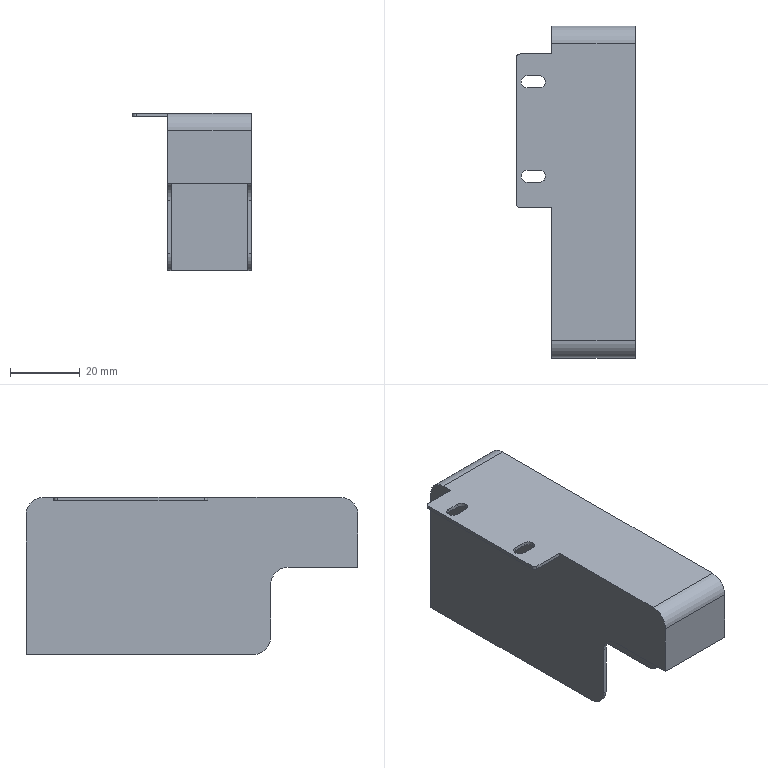Part | STEP file | 11-FG-B01211 | 1 solid | 38 faces | box 34 x 95 x 45 mm | volume 11150 mm3 | plane 22 | cylinder 16 | commonest cylinder face diameters 10 x8 3.5 x6 2 x2
STEP:
#1=CARTESIAN_POINT('',(-13.75,4.5,44.));
#2=VERTEX_POINT('',#1);
#3=CARTESIAN_POINT('',(-15.5,6.25,44.));
#4=VERTEX_POINT('',#3);
#5=CARTESIAN_POINT('',(-15.5,4.5,44.));
#6=DIRECTION('',(0.,0.,1.));
#7=DIRECTION('',(1.,0.,0.));
#8=AXIS2_PLACEMENT_3D('',#5,#6,#7);
#9=CIRCLE('',#8,1.75);
#10=EDGE_CURVE('',#2,#4,#9,.T.);
#11=ORIENTED_EDGE('',*,*,#10,.F.);
#12=CARTESIAN_POINT('',(-13.75,4.5,45.));
#13=VERTEX_POINT('',#12);
#14=CARTESIAN_POINT('',(-13.75,4.5,-20.));
#15=DIRECTION('',(0.,0.,1.));
#16=VECTOR('',#15,1000.);
#17=LINE('',#14,#16);
#18=EDGE_CURVE('',#2,#13,#17,.T.);
#19=ORIENTED_EDGE('',*,*,#18,.T.);
#20=CARTESIAN_POINT('',(-15.5,6.25,45.));
#21=VERTEX_POINT('',#20);
#22=CARTESIAN_POINT('',(-15.5,4.5,45.));
#23=DIRECTION('',(0.,0.,1.));
#24=DIRECTION('',(1.,0.,0.));
#25=AXIS2_PLACEMENT_3D('',#22,#23,#24);
#26=CIRCLE('',#25,1.75);
#27=EDGE_CURVE('',#13,#21,#26,.T.);
#28=ORIENTED_EDGE('',*,*,#27,.T.);
#29=CARTESIAN_POINT('',(-15.5,6.25,-20.));
#30=DIRECTION('',(0.,0.,1.));
#31=VECTOR('',#30,1000.);
#32=LINE('',#29,#31);
#33=EDGE_CURVE('',#4,#21,#32,.T.);
#34=ORIENTED_EDGE('',*,*,#33,.F.);
#35=EDGE_LOOP('',(#11,#19,#28,#34));
#36=FACE_OUTER_BOUND('',#35,.T.);
#37=CARTESIAN_POINT('',(-15.5,4.5,-20.));
#38=DIRECTION('',(0.,0.,1.));
#39=DIRECTION('',(1.,0.,0.));
#40=AXIS2_PLACEMENT_3D('',#37,#38,#39);
#41=CYLINDRICAL_SURFACE('',#40,1.75);
#42=ADVANCED_FACE('',(#36),#41,.F.);
#43=CARTESIAN_POINT('',(-13.75,31.5,44.));
#44=VERTEX_POINT('',#43);
#45=CARTESIAN_POINT('',(-15.5,33.25,44.));
#46=VERTEX_POINT('',#45);
#47=CARTESIAN_POINT('',(-15.5,31.5,44.));
#48=DIRECTION('',(0.,0.,1.));
#49=DIRECTION('',(1.,0.,0.));
#50=AXIS2_PLACEMENT_3D('',#47,#48,#49);
#51=CIRCLE('',#50,1.75);
#52=EDGE_CURVE('',#44,#46,#51,.T.);
#53=ORIENTED_EDGE('',*,*,#52,.F.);
#54=CARTESIAN_POINT('',(-13.75,31.5,45.));
#55=VERTEX_POINT('',#54);
#56=CARTESIAN_POINT('',(-13.75,31.5,-20.));
#57=DIRECTION('',(0.,0.,1.));
#58=VECTOR('',#57,1000.);
#59=LINE('',#56,#58);
#60=EDGE_CURVE('',#44,#55,#59,.T.);
#61=ORIENTED_EDGE('',*,*,#60,.T.);
#62=CARTESIAN_POINT('',(-15.5,33.25,45.));
#63=VERTEX_POINT('',#62);
#64=CARTESIAN_POINT('',(-15.5,31.5,45.));
#65=DIRECTION('',(0.,0.,1.));
#66=DIRECTION('',(1.,0.,0.));
#67=AXIS2_PLACEMENT_3D('',#64,#65,#66);
#68=CIRCLE('',#67,1.75);
#69=EDGE_CURVE('',#55,#63,#68,.T.);
#70=ORIENTED_EDGE('',*,*,#69,.T.);
#71=CARTESIAN_POINT('',(-15.5,33.25,-20.));
#72=DIRECTION('',(0.,0.,1.));
#73=VECTOR('',#72,1000.);
#74=LINE('',#71,#73);
#75=EDGE_CURVE('',#46,#63,#74,.T.);
#76=ORIENTED_EDGE('',*,*,#75,.F.);
#77=EDGE_LOOP('',(#53,#61,#70,#76));
#78=FACE_OUTER_BOUND('',#77,.T.);
#79=CARTESIAN_POINT('',(-15.5,31.5,-20.));
#80=DIRECTION('',(0.,0.,1.));
#81=DIRECTION('',(1.,0.,0.));
#82=AXIS2_PLACEMENT_3D('',#79,#80,#81);
#83=CYLINDRICAL_SURFACE('',#82,1.75);
#84=ADVANCED_FACE('',(#78),#83,.F.);
#85=CARTESIAN_POINT('',(-12.,47.5,0.));
#86=VERTEX_POINT('',#85);
#87=CARTESIAN_POINT('',(-12.,-17.5,0.));
#88=VERTEX_POINT('',#87);
#89=CARTESIAN_POINT('',(-12.,47.5,0.));
#90=DIRECTION('',(0.,-1.,0.));
#91=VECTOR('',#90,1000.);
#92=LINE('',#89,#91);
#93=EDGE_CURVE('',#86,#88,#92,.T.);
#94=ORIENTED_EDGE('',*,*,#93,.T.);
#95=CARTESIAN_POINT('',(-12.,-22.5,5.));
#96=VERTEX_POINT('',#95);
#97=CARTESIAN_POINT('',(-12.,-17.5,5.));
#98=DIRECTION('',(-1.,0.,0.));
#99=DIRECTION('',(0.,1.,0.));
#100=AXIS2_PLACEMENT_3D('',#97,#98,#99);
#101=CIRCLE('',#100,5.);
#102=EDGE_CURVE('',#88,#96,#101,.T.);
#103=ORIENTED_EDGE('',*,*,#102,.T.);
#104=CARTESIAN_POINT('',(-12.,-22.5,20.));
#105=VERTEX_POINT('',#104);
#106=CARTESIAN_POINT('',(-12.,-22.5,0.));
#107=DIRECTION('',(0.,0.,-1.));
#108=VECTOR('',#107,1000.);
#109=LINE('',#106,#108);
#110=EDGE_CURVE('',#105,#96,#109,.T.);
#111=ORIENTED_EDGE('',*,*,#110,.F.);
#112=CARTESIAN_POINT('',(-12.,-27.5,25.));
#113=VERTEX_POINT('',#112);
#114=CARTESIAN_POINT('',(-12.,-27.5,20.));
#115=DIRECTION('',(1.,0.,0.));
#116=DIRECTION('',(0.,1.,0.));
#117=AXIS2_PLACEMENT_3D('',#114,#115,#116);
#118=CIRCLE('',#117,5.);
#119=EDGE_CURVE('',#105,#113,#118,.T.);
#120=ORIENTED_EDGE('',*,*,#119,.T.);
#121=CARTESIAN_POINT('',(-12.,-47.5,25.));
#122=VERTEX_POINT('',#121);
#123=CARTESIAN_POINT('',(-12.,-47.5,25.));
#124=DIRECTION('',(0.,1.,0.));
#125=VECTOR('',#124,1000.);
#126=LINE('',#123,#125);
#127=EDGE_CURVE('',#122,#113,#126,.T.);
#128=ORIENTED_EDGE('',*,*,#127,.F.);
#129=CARTESIAN_POINT('',(-12.,-47.5,40.));
#130=VERTEX_POINT('',#129);
#131=CARTESIAN_POINT('',(-12.,-47.5,45.));
#132=DIRECTION('',(0.,0.,-1.));
#133=VECTOR('',#132,1000.);
#134=LINE('',#131,#133);
#135=EDGE_CURVE('',#130,#122,#134,.T.);
#136=ORIENTED_EDGE('',*,*,#135,.F.);
#137=CARTESIAN_POINT('',(-12.,-42.5,45.));
#138=VERTEX_POINT('',#137);
#139=CARTESIAN_POINT('',(-12.,-42.5,40.));
#140=DIRECTION('',(-1.,0.,0.));
#141=DIRECTION('',(0.,1.,0.));
#142=AXIS2_PLACEMENT_3D('',#139,#140,#141);
#143=CIRCLE('',#142,5.);
#144=EDGE_CURVE('',#130,#138,#143,.T.);
#145=ORIENTED_EDGE('',*,*,#144,.T.);
#146=CARTESIAN_POINT('',(-12.,-4.5,45.));
#147=VERTEX_POINT('',#146);
#148=CARTESIAN_POINT('',(-12.,47.5,45.));
#149=DIRECTION('',(0.,-1.,0.));
#150=VECTOR('',#149,1000.);
#151=LINE('',#148,#150);
#152=EDGE_CURVE('',#147,#138,#151,.T.);
#153=ORIENTED_EDGE('',*,*,#152,.F.);
#154=CARTESIAN_POINT('',(-12.,-4.5,44.));
#155=VERTEX_POINT('',#154);
#156=CARTESIAN_POINT('',(-12.,-4.5,-20.));
#157=DIRECTION('',(0.,0.,1.));
#158=VECTOR('',#157,1000.);
#159=LINE('',#156,#158);
#160=EDGE_CURVE('',#155,#147,#159,.T.);
#161=ORIENTED_EDGE('',*,*,#160,.F.);
#162=CARTESIAN_POINT('',(-12.,39.5,44.));
#163=VERTEX_POINT('',#162);
#164=CARTESIAN_POINT('',(-12.,47.5,44.));
#165=DIRECTION('',(0.,-1.,0.));
#166=VECTOR('',#165,1000.);
#167=LINE('',#164,#166);
#168=EDGE_CURVE('',#163,#155,#167,.T.);
#169=ORIENTED_EDGE('',*,*,#168,.F.);
#170=CARTESIAN_POINT('',(-12.,39.5,45.));
#171=VERTEX_POINT('',#170);
#172=CARTESIAN_POINT('',(-12.,39.5,109.));
#173=DIRECTION('',(0.,0.,-1.));
#174=VECTOR('',#173,1000.);
#175=LINE('',#172,#174);
#176=EDGE_CURVE('',#171,#163,#175,.T.);
#177=ORIENTED_EDGE('',*,*,#176,.F.);
#178=CARTESIAN_POINT('',(-12.,42.5,45.));
#179=VERTEX_POINT('',#178);
#180=CARTESIAN_POINT('',(-12.,0.,45.));
#181=DIRECTION('',(0.,1.,0.));
#182=VECTOR('',#181,1000.);
#183=LINE('',#180,#182);
#184=EDGE_CURVE('',#171,#179,#183,.T.);
#185=ORIENTED_EDGE('',*,*,#184,.T.);
#186=CARTESIAN_POINT('',(-12.,47.5,40.));
#187=VERTEX_POINT('',#186);
#188=CARTESIAN_POINT('',(-12.,42.5,40.));
#189=DIRECTION('',(-1.,0.,0.));
#190=DIRECTION('',(0.,1.,0.));
#191=AXIS2_PLACEMENT_3D('',#188,#189,#190);
#192=CIRCLE('',#191,5.);
#193=EDGE_CURVE('',#179,#187,#192,.T.);
#194=ORIENTED_EDGE('',*,*,#193,.T.);
#195=CARTESIAN_POINT('',(-12.,47.5,45.));
#196=DIRECTION('',(0.,0.,-1.));
#197=VECTOR('',#196,1000.);
#198=LINE('',#195,#197);
#199=EDGE_CURVE('',#187,#86,#198,.T.);
#200=ORIENTED_EDGE('',*,*,#199,.T.);
#201=EDGE_LOOP('',(#94,#103,#111,#120,#128,#136,#145,#153,#161,#169,#177,#185,#194,#200));
#202=FACE_OUTER_BOUND('',#201,.T.);
#203=CARTESIAN_POINT('',(-12.,47.5,45.));
#204=DIRECTION('',(1.,0.,0.));
#205=DIRECTION('',(0.,1.,0.));
#206=AXIS2_PLACEMENT_3D('',#203,#204,#205);
#207=PLANE('',#206);
#208=ADVANCED_FACE('',(#202),#207,.F.);
#209=CARTESIAN_POINT('',(12.,-22.5,20.));
#210=VERTEX_POINT('',#209);
#211=CARTESIAN_POINT('',(12.,-22.5,5.));
#212=VERTEX_POINT('',#211);
#213=CARTESIAN_POINT('',(12.,-22.5,45.));
#214=DIRECTION('',(0.,0.,-1.));
#215=VECTOR('',#214,1000.);
#216=LINE('',#213,#215);
#217=EDGE_CURVE('',#210,#212,#216,.T.);
#218=ORIENTED_EDGE('',*,*,#217,.T.);
#219=CARTESIAN_POINT('',(12.,-17.5,0.));
#220=VERTEX_POINT('',#219);
#221=CARTESIAN_POINT('',(12.,-17.5,5.));
#222=DIRECTION('',(1.,0.,0.));
#223=DIRECTION('',(0.,-1.,0.));
#224=AXIS2_PLACEMENT_3D('',#221,#222,#223);
#225=CIRCLE('',#224,5.);
#226=EDGE_CURVE('',#212,#220,#225,.T.);
#227=ORIENTED_EDGE('',*,*,#226,.T.);
#228=CARTESIAN_POINT('',(12.,47.5,0.));
#229=VERTEX_POINT('',#228);
#230=CARTESIAN_POINT('',(12.,47.5,0.));
#231=DIRECTION('',(0.,1.,0.));
#232=VECTOR('',#231,1000.);
#233=LINE('',#230,#232);
#234=EDGE_CURVE('',#220,#229,#233,.T.);
#235=ORIENTED_EDGE('',*,*,#234,.T.);
#236=CARTESIAN_POINT('',(12.,47.5,40.));
#237=VERTEX_POINT('',#236);
#238=CARTESIAN_POINT('',(12.,47.5,45.));
#239=DIRECTION('',(0.,0.,-1.));
#240=VECTOR('',#239,1000.);
#241=LINE('',#238,#240);
#242=EDGE_CURVE('',#237,#229,#241,.T.);
#243=ORIENTED_EDGE('',*,*,#242,.F.);
#244=CARTESIAN_POINT('',(12.,42.5,45.));
#245=VERTEX_POINT('',#244);
#246=CARTESIAN_POINT('',(12.,42.5,40.));
#247=DIRECTION('',(1.,0.,0.));
#248=DIRECTION('',(0.,-1.,0.));
#249=AXIS2_PLACEMENT_3D('',#246,#247,#248);
#250=CIRCLE('',#249,5.);
#251=EDGE_CURVE('',#237,#245,#250,.T.);
#252=ORIENTED_EDGE('',*,*,#251,.T.);
#253=CARTESIAN_POINT('',(12.,-42.5,45.));
#254=VERTEX_POINT('',#253);
#255=CARTESIAN_POINT('',(12.,47.5,45.));
#256=DIRECTION('',(0.,1.,0.));
#257=VECTOR('',#256,1000.);
#258=LINE('',#255,#257);
#259=EDGE_CURVE('',#254,#245,#258,.T.);
#260=ORIENTED_EDGE('',*,*,#259,.F.);
#261=CARTESIAN_POINT('',(12.,-47.5,40.));
#262=VERTEX_POINT('',#261);
#263=CARTESIAN_POINT('',(12.,-42.5,40.));
#264=DIRECTION('',(1.,0.,0.));
#265=DIRECTION('',(0.,-1.,0.));
#266=AXIS2_PLACEMENT_3D('',#263,#264,#265);
#267=CIRCLE('',#266,5.);
#268=EDGE_CURVE('',#254,#262,#267,.T.);
#269=ORIENTED_EDGE('',*,*,#268,.T.);
#270=CARTESIAN_POINT('',(12.,-47.5,25.));
#271=VERTEX_POINT('',#270);
#272=CARTESIAN_POINT('',(12.,-47.5,45.));
#273=DIRECTION('',(0.,0.,-1.));
#274=VECTOR('',#273,1000.);
#275=LINE('',#272,#274);
#276=EDGE_CURVE('',#262,#271,#275,.T.);
#277=ORIENTED_EDGE('',*,*,#276,.T.);
#278=CARTESIAN_POINT('',(12.,-27.5,25.));
#279=VERTEX_POINT('',#278);
#280=CARTESIAN_POINT('',(12.,47.5,25.));
#281=DIRECTION('',(0.,1.,0.));
#282=VECTOR('',#281,1000.);
#283=LINE('',#280,#282);
#284=EDGE_CURVE('',#271,#279,#283,.T.);
#285=ORIENTED_EDGE('',*,*,#284,.T.);
#286=CARTESIAN_POINT('',(12.,-27.5,20.));
#287=DIRECTION('',(-1.,0.,0.));
#288=DIRECTION('',(0.,-1.,0.));
#289=AXIS2_PLACEMENT_3D('',#286,#287,#288);
#290=CIRCLE('',#289,5.);
#291=EDGE_CURVE('',#279,#210,#290,.T.);
#292=ORIENTED_EDGE('',*,*,#291,.T.);
#293=EDGE_LOOP('',(#218,#227,#235,#243,#252,#260,#269,#277,#285,#292));
#294=FACE_OUTER_BOUND('',#293,.T.);
#295=CARTESIAN_POINT('',(12.,47.5,45.));
#296=DIRECTION('',(-1.,0.,0.));
#297=DIRECTION('',(0.,-1.,0.));
#298=AXIS2_PLACEMENT_3D('',#295,#296,#297);
#299=PLANE('',#298);
#300=ADVANCED_FACE('',(#294),#299,.F.);
#301=ORIENTED_EDGE('',*,*,#199,.F.);
#302=CARTESIAN_POINT('',(12.,47.5,40.));
#303=DIRECTION('',(1.,0.,0.));
#304=VECTOR('',#303,1000.);
#305=LINE('',#302,#304);
#306=EDGE_CURVE('',#187,#237,#305,.T.);
#307=ORIENTED_EDGE('',*,*,#306,.T.);
#308=ORIENTED_EDGE('',*,*,#242,.T.);
#309=CARTESIAN_POINT('',(-12.,47.5,0.));
#310=DIRECTION('',(-1.,0.,0.));
#311=VECTOR('',#310,1000.);
#312=LINE('',#309,#311);
#313=EDGE_CURVE('',#229,#86,#312,.T.);
#314=ORIENTED_EDGE('',*,*,#313,.T.);
#315=EDGE_LOOP('',(#301,#307,#308,#314));
#316=FACE_OUTER_BOUND('',#315,.T.);
#317=CARTESIAN_POINT('',(-12.,47.5,45.));
#318=DIRECTION('',(0.,-1.,0.));
#319=DIRECTION('',(0.,0.,-1.));
#320=AXIS2_PLACEMENT_3D('',#317,#318,#319);
#321=PLANE('',#320);
#322=ADVANCED_FACE('',(#316),#321,.F.);
#323=ORIENTED_EDGE('',*,*,#135,.T.);
#324=CARTESIAN_POINT('',(53.,-47.5,25.));
#325=DIRECTION('',(-1.,0.,0.));
#326=VECTOR('',#325,1000.);
#327=LINE('',#324,#326);
#328=EDGE_CURVE('',#271,#122,#327,.T.);
#329=ORIENTED_EDGE('',*,*,#328,.F.);
#330=ORIENTED_EDGE('',*,*,#276,.F.);
#331=CARTESIAN_POINT('',(-12.,-47.5,40.));
#332=DIRECTION('',(-1.,0.,0.));
#333=VECTOR('',#332,1000.);
#334=LINE('',#331,#333);
#335=EDGE_CURVE('',#262,#130,#334,.T.);
#336=ORIENTED_EDGE('',*,*,#335,.T.);
#337=EDGE_LOOP('',(#323,#329,#330,#336));
#338=FACE_OUTER_BOUND('',#337,.T.);
#339=CARTESIAN_POINT('',(-12.,-47.5,45.));
#340=DIRECTION('',(0.,1.,0.));
#341=DIRECTION('',(0.,0.,1.));
#342=AXIS2_PLACEMENT_3D('',#339,#340,#341);
#343=PLANE('',#342);
#344=ADVANCED_FACE('',(#338),#343,.F.);
#345=CARTESIAN_POINT('',(-22.,38.5,45.));
#346=VERTEX_POINT('',#345);
#347=CARTESIAN_POINT('',(-22.,-3.5,45.));
#348=VERTEX_POINT('',#347);
#349=CARTESIAN_POINT('',(-22.,47.5,45.));
#350=DIRECTION('',(0.,-1.,0.));
#351=VECTOR('',#350,1000.);
#352=LINE('',#349,#351);
#353=EDGE_CURVE('',#346,#348,#352,.T.);
#354=ORIENTED_EDGE('',*,*,#353,.T.);
#355=CARTESIAN_POINT('',(-21.,-4.5,45.));
#356=VERTEX_POINT('',#355);
#357=CARTESIAN_POINT('',(-21.,-3.5,45.));
#358=DIRECTION('',(0.,0.,1.));
#359=DIRECTION('',(1.,0.,0.));
#360=AXIS2_PLACEMENT_3D('',#357,#358,#359);
#361=CIRCLE('',#360,1.);
#362=EDGE_CURVE('',#348,#356,#361,.T.);
#363=ORIENTED_EDGE('',*,*,#362,.T.);
#364=CARTESIAN_POINT('',(-12.,-4.5,45.));
#365=DIRECTION('',(-1.,0.,0.));
#366=VECTOR('',#365,1000.);
#367=LINE('',#364,#366);
#368=EDGE_CURVE('',#147,#356,#367,.T.);
#369=ORIENTED_EDGE('',*,*,#368,.F.);
#370=ORIENTED_EDGE('',*,*,#152,.T.);
#371=CARTESIAN_POINT('',(12.,-42.5,45.));
#372=DIRECTION('',(1.,0.,0.));
#373=VECTOR('',#372,1000.);
#374=LINE('',#371,#373);
#375=EDGE_CURVE('',#138,#254,#374,.T.);
#376=ORIENTED_EDGE('',*,*,#375,.T.);
#377=ORIENTED_EDGE('',*,*,#259,.T.);
#378=CARTESIAN_POINT('',(-22.,42.5,45.));
#379=DIRECTION('',(-1.,0.,0.));
#380=VECTOR('',#379,1000.);
#381=LINE('',#378,#380);
#382=EDGE_CURVE('',#245,#179,#381,.T.);
#383=ORIENTED_EDGE('',*,*,#382,.T.);
#384=ORIENTED_EDGE('',*,*,#184,.F.);
#385=CARTESIAN_POINT('',(-21.,39.5,45.));
#386=VERTEX_POINT('',#385);
#387=CARTESIAN_POINT('',(0.,39.5,45.));
#388=DIRECTION('',(1.,0.,0.));
#389=VECTOR('',#388,1000.);
#390=LINE('',#387,#389);
#391=EDGE_CURVE('',#386,#171,#390,.T.);
#392=ORIENTED_EDGE('',*,*,#391,.F.);
#393=CARTESIAN_POINT('',(-21.,38.5,45.));
#394=DIRECTION('',(0.,0.,1.));
#395=DIRECTION('',(1.,0.,0.));
#396=AXIS2_PLACEMENT_3D('',#393,#394,#395);
#397=CIRCLE('',#396,1.);
#398=EDGE_CURVE('',#386,#346,#397,.T.);
#399=ORIENTED_EDGE('',*,*,#398,.T.);
#400=EDGE_LOOP('',(#354,#363,#369,#370,#376,#377,#383,#384,#392,#399));
#401=FACE_OUTER_BOUND('',#400,.T.);
#402=CARTESIAN_POINT('',(-19.,6.25,45.));
#403=VERTEX_POINT('',#402);
#404=CARTESIAN_POINT('',(-19.,2.75,45.));
#405=VERTEX_POINT('',#404);
#406=CARTESIAN_POINT('',(-19.,4.5,45.));
#407=DIRECTION('',(0.,0.,1.));
#408=DIRECTION('',(1.,0.,0.));
#409=AXIS2_PLACEMENT_3D('',#406,#407,#408);
#410=CIRCLE('',#409,1.75);
#411=EDGE_CURVE('',#403,#405,#410,.T.);
#412=ORIENTED_EDGE('',*,*,#411,.F.);
#413=CARTESIAN_POINT('',(-19.,6.25,45.));
#414=DIRECTION('',(-1.,0.,0.));
#415=VECTOR('',#414,1000.);
#416=LINE('',#413,#415);
#417=EDGE_CURVE('',#21,#403,#416,.T.);
#418=ORIENTED_EDGE('',*,*,#417,.F.);
#419=ORIENTED_EDGE('',*,*,#27,.F.);
#420=CARTESIAN_POINT('',(-15.5,2.75,45.));
#421=VERTEX_POINT('',#420);
#422=CARTESIAN_POINT('',(-15.5,4.5,45.));
#423=DIRECTION('',(0.,0.,1.));
#424=DIRECTION('',(1.,0.,0.));
#425=AXIS2_PLACEMENT_3D('',#422,#423,#424);
#426=CIRCLE('',#425,1.75);
#427=EDGE_CURVE('',#421,#13,#426,.T.);
#428=ORIENTED_EDGE('',*,*,#427,.F.);
#429=CARTESIAN_POINT('',(-19.,2.75,45.));
#430=DIRECTION('',(1.,0.,0.));
#431=VECTOR('',#430,1000.);
#432=LINE('',#429,#431);
#433=EDGE_CURVE('',#405,#421,#432,.T.);
#434=ORIENTED_EDGE('',*,*,#433,.F.);
#435=EDGE_LOOP('',(#412,#418,#419,#428,#434));
#436=FACE_BOUND('',#435,.T.);
#437=CARTESIAN_POINT('',(-19.,33.25,45.));
#438=VERTEX_POINT('',#437);
#439=CARTESIAN_POINT('',(-19.,29.75,45.));
#440=VERTEX_POINT('',#439);
#441=CARTESIAN_POINT('',(-19.,31.5,45.));
#442=DIRECTION('',(0.,0.,1.));
#443=DIRECTION('',(1.,0.,0.));
#444=AXIS2_PLACEMENT_3D('',#441,#442,#443);
#445=CIRCLE('',#444,1.75);
#446=EDGE_CURVE('',#438,#440,#445,.T.);
#447=ORIENTED_EDGE('',*,*,#446,.F.);
#448=CARTESIAN_POINT('',(-19.,33.25,45.));
#449=DIRECTION('',(-1.,0.,0.));
#450=VECTOR('',#449,1000.);
#451=LINE('',#448,#450);
#452=EDGE_CURVE('',#63,#438,#451,.T.);
#453=ORIENTED_EDGE('',*,*,#452,.F.);
#454=ORIENTED_EDGE('',*,*,#69,.F.);
#455=CARTESIAN_POINT('',(-15.5,29.75,45.));
#456=VERTEX_POINT('',#455);
#457=CARTESIAN_POINT('',(-15.5,31.5,45.));
#458=DIRECTION('',(0.,0.,1.));
#459=DIRECTION('',(1.,0.,0.));
#460=AXIS2_PLACEMENT_3D('',#457,#458,#459);
#461=CIRCLE('',#460,1.75);
#462=EDGE_CURVE('',#456,#55,#461,.T.);
#463=ORIENTED_EDGE('',*,*,#462,.F.);
#464=CARTESIAN_POINT('',(-19.,29.75,45.));
#465=DIRECTION('',(1.,0.,0.));
#466=VECTOR('',#465,1000.);
#467=LINE('',#464,#466);
#468=EDGE_CURVE('',#440,#456,#467,.T.);
#469=ORIENTED_EDGE('',*,*,#468,.F.);
#470=EDGE_LOOP('',(#447,#453,#454,#463,#469));
#471=FACE_BOUND('',#470,.T.);
#472=CARTESIAN_POINT('',(0.,0.,45.));
#473=DIRECTION('',(0.,0.,1.));
#474=DIRECTION('',(1.,0.,0.));
#475=AXIS2_PLACEMENT_3D('',#472,#473,#474);
#476=PLANE('',#475);
#477=ADVANCED_FACE('',(#401,#436,#471),#476,.T.);
#478=ORIENTED_EDGE('',*,*,#234,.F.);
#479=CARTESIAN_POINT('',(11.,-17.5,0.));
#480=VERTEX_POINT('',#479);
#481=CARTESIAN_POINT('',(0.,-17.5,0.));
#482=DIRECTION('',(-1.,0.,0.));
#483=VECTOR('',#482,1000.);
#484=LINE('',#481,#483);
#485=EDGE_CURVE('',#220,#480,#484,.T.);
#486=ORIENTED_EDGE('',*,*,#485,.T.);
#487=CARTESIAN_POINT('',(11.,46.5,0.));
#488=VERTEX_POINT('',#487);
#489=CARTESIAN_POINT('',(11.,47.5,0.));
#490=DIRECTION('',(0.,1.,0.));
#491=VECTOR('',#490,1000.);
#492=LINE('',#489,#491);
#493=EDGE_CURVE('',#480,#488,#492,.T.);
#494=ORIENTED_EDGE('',*,*,#493,.T.);
#495=CARTESIAN_POINT('',(-11.,46.5,0.));
#496=VERTEX_POINT('',#495);
#497=CARTESIAN_POINT('',(-12.,46.5,0.));
#498=DIRECTION('',(-1.,0.,0.));
#499=VECTOR('',#498,1000.);
#500=LINE('',#497,#499);
#501=EDGE_CURVE('',#488,#496,#500,.T.);
#502=ORIENTED_EDGE('',*,*,#501,.T.);
#503=CARTESIAN_POINT('',(-11.,-17.5,0.));
#504=VERTEX_POINT('',#503);
#505=CARTESIAN_POINT('',(-11.,47.5,0.));
#506=DIRECTION('',(0.,-1.,0.));
#507=VECTOR('',#506,1000.);
#508=LINE('',#505,#507);
#509=EDGE_CURVE('',#496,#504,#508,.T.);
#510=ORIENTED_EDGE('',*,*,#509,.T.);
#511=CARTESIAN_POINT('',(0.,-17.5,0.));
#512=DIRECTION('',(-1.,0.,0.));
#513=VECTOR('',#512,1000.);
#514=LINE('',#511,#513);
#515=EDGE_CURVE('',#504,#88,#514,.T.);
#516=ORIENTED_EDGE('',*,*,#515,.T.);
#517=ORIENTED_EDGE('',*,*,#93,.F.);
#518=ORIENTED_EDGE('',*,*,#313,.F.);
#519=EDGE_LOOP('',(#478,#486,#494,#502,#510,#516,#517,#518));
#520=FACE_OUTER_BOUND('',#519,.T.);
#521=CARTESIAN_POINT('',(0.,0.,0.));
#522=DIRECTION('',(0.,0.,1.));
#523=DIRECTION('',(1.,0.,0.));
#524=AXIS2_PLACEMENT_3D('',#521,#522,#523);
#525=PLANE('',#524);
#526=ADVANCED_FACE('',(#520),#525,.F.);
#527=ORIENTED_EDGE('',*,*,#493,.F.);
#528=CARTESIAN_POINT('',(11.,-22.5,5.));
#529=VERTEX_POINT('',#528);
#530=CARTESIAN_POINT('',(11.,-17.5,5.));
#531=DIRECTION('',(-1.,0.,0.));
#532=DIRECTION('',(0.,-1.,0.));
#533=AXIS2_PLACEMENT_3D('',#530,#531,#532);
#534=CIRCLE('',#533,5.);
#535=EDGE_CURVE('',#480,#529,#534,.T.);
#536=ORIENTED_EDGE('',*,*,#535,.T.);
#537=CARTESIAN_POINT('',(11.,-22.5,20.));
#538=VERTEX_POINT('',#537);
#539=CARTESIAN_POINT('',(11.,-22.5,45.));
#540=DIRECTION('',(0.,0.,-1.));
#541=VECTOR('',#540,1000.);
#542=LINE('',#539,#541);
#543=EDGE_CURVE('',#538,#529,#542,.T.);
#544=ORIENTED_EDGE('',*,*,#543,.F.);
#545=CARTESIAN_POINT('',(11.,-27.5,25.));
#546=VERTEX_POINT('',#545);
#547=CARTESIAN_POINT('',(11.,-27.5,20.));
#548=DIRECTION('',(1.,0.,0.));
#549=DIRECTION('',(0.,-1.,0.));
#550=AXIS2_PLACEMENT_3D('',#547,#548,#549);
#551=CIRCLE('',#550,5.);
#552=EDGE_CURVE('',#538,#546,#551,.T.);
#553=ORIENTED_EDGE('',*,*,#552,.T.);
#554=CARTESIAN_POINT('',(11.,-46.5,25.));
#555=VERTEX_POINT('',#554);
#556=CARTESIAN_POINT('',(11.,47.5,25.));
#557=DIRECTION('',(0.,1.,0.));
#558=VECTOR('',#557,1000.);
#559=LINE('',#556,#558);
#560=EDGE_CURVE('',#555,#546,#559,.T.);
#561=ORIENTED_EDGE('',*,*,#560,.F.);
#562=CARTESIAN_POINT('',(11.,-46.5,39.));
#563=VERTEX_POINT('',#562);
#564=CARTESIAN_POINT('',(11.,-46.5,45.));
#565=DIRECTION('',(0.,0.,-1.));
#566=VECTOR('',#565,1000.);
#567=LINE('',#564,#566);
#568=EDGE_CURVE('',#563,#555,#567,.T.);
#569=ORIENTED_EDGE('',*,*,#568,.F.);
#570=CARTESIAN_POINT('',(11.,-41.5,44.));
#571=VERTEX_POINT('',#570);
#572=CARTESIAN_POINT('',(11.,-41.5,39.));
#573=DIRECTION('',(-1.,0.,0.));
#574=DIRECTION('',(0.,-1.,0.));
#575=AXIS2_PLACEMENT_3D('',#572,#573,#574);
#576=CIRCLE('',#575,5.);
#577=EDGE_CURVE('',#563,#571,#576,.T.);
#578=ORIENTED_EDGE('',*,*,#577,.T.);
#579=CARTESIAN_POINT('',(11.,41.5,44.));
#580=VERTEX_POINT('',#579);
#581=CARTESIAN_POINT('',(11.,47.5,44.));
#582=DIRECTION('',(0.,1.,0.));
#583=VECTOR('',#582,1000.);
#584=LINE('',#581,#583);
#585=EDGE_CURVE('',#571,#580,#584,.T.);
#586=ORIENTED_EDGE('',*,*,#585,.T.);
#587=CARTESIAN_POINT('',(11.,46.5,39.));
#588=VERTEX_POINT('',#587);
#589=CARTESIAN_POINT('',(11.,41.5,39.));
#590=DIRECTION('',(-1.,0.,0.));
#591=DIRECTION('',(0.,-1.,0.));
#592=AXIS2_PLACEMENT_3D('',#589,#590,#591);
#593=CIRCLE('',#592,5.);
#594=EDGE_CURVE('',#580,#588,#593,.T.);
#595=ORIENTED_EDGE('',*,*,#594,.T.);
#596=CARTESIAN_POINT('',(11.,46.5,45.));
#597=DIRECTION('',(0.,0.,-1.));
#598=VECTOR('',#597,1000.);
#599=LINE('',#596,#598);
#600=EDGE_CURVE('',#588,#488,#599,.T.);
#601=ORIENTED_EDGE('',*,*,#600,.T.);
#602=EDGE_LOOP('',(#527,#536,#544,#553,#561,#569,#578,#586,#595,#601));
#603=FACE_OUTER_BOUND('',#602,.T.);
#604=CARTESIAN_POINT('',(11.,47.5,45.));
#605=DIRECTION('',(-1.,0.,0.));
#606=DIRECTION('',(0.,-1.,0.));
#607=AXIS2_PLACEMENT_3D('',#604,#605,#606);
#608=PLANE('',#607);
#609=ADVANCED_FACE('',(#603),#608,.T.);
#610=ORIENTED_EDGE('',*,*,#600,.F.);
#611=CARTESIAN_POINT('',(-11.,46.5,39.));
#612=VERTEX_POINT('',#611);
#613=CARTESIAN_POINT('',(-12.,46.5,39.));
#614=DIRECTION('',(-1.,0.,0.));
#615=VECTOR('',#614,1000.);
#616=LINE('',#613,#615);
#617=EDGE_CURVE('',#588,#612,#616,.T.);
#618=ORIENTED_EDGE('',*,*,#617,.T.);
#619=CARTESIAN_POINT('',(-11.,46.5,45.));
#620=DIRECTION('',(0.,0.,-1.));
#621=VECTOR('',#620,1000.);
#622=LINE('',#619,#621);
#623=EDGE_CURVE('',#612,#496,#622,.T.);
#624=ORIENTED_EDGE('',*,*,#623,.T.);
#625=ORIENTED_EDGE('',*,*,#501,.F.);
#626=EDGE_LOOP('',(#610,#618,#624,#625));
#627=FACE_OUTER_BOUND('',#626,.T.);
#628=CARTESIAN_POINT('',(-12.,46.5,45.));
#629=DIRECTION('',(0.,-1.,0.));
#630=DIRECTION('',(0.,0.,-1.));
#631=AXIS2_PLACEMENT_3D('',#628,#629,#630);
#632=PLANE('',#631);
#633=ADVANCED_FACE('',(#627),#632,.T.);
#634=CARTESIAN_POINT('',(-11.,-22.5,5.));
#635=VERTEX_POINT('',#634);
#636=CARTESIAN_POINT('',(-11.,-22.5,20.));
#637=VERTEX_POINT('',#636);
#638=CARTESIAN_POINT('',(-11.,-22.5,45.));
#639=DIRECTION('',(0.,0.,1.));
#640=VECTOR('',#639,1000.);
#641=LINE('',#638,#640);
#642=EDGE_CURVE('',#635,#637,#641,.T.);
#643=ORIENTED_EDGE('',*,*,#642,.F.);
#644=CARTESIAN_POINT('',(-11.,-17.5,5.));
#645=DIRECTION('',(1.,0.,0.));
#646=DIRECTION('',(0.,1.,0.));
#647=AXIS2_PLACEMENT_3D('',#644,#645,#646);
#648=CIRCLE('',#647,5.);
#649=EDGE_CURVE('',#635,#504,#648,.T.);
#650=ORIENTED_EDGE('',*,*,#649,.T.);
#651=ORIENTED_EDGE('',*,*,#509,.F.);
#652=ORIENTED_EDGE('',*,*,#623,.F.);
#653=CARTESIAN_POINT('',(-11.,41.5,44.));
#654=VERTEX_POINT('',#653);
#655=CARTESIAN_POINT('',(-11.,41.5,39.));
#656=DIRECTION('',(1.,0.,0.));
#657=DIRECTION('',(0.,1.,0.));
#658=AXIS2_PLACEMENT_3D('',#655,#656,#657);
#659=CIRCLE('',#658,5.);
#660=EDGE_CURVE('',#612,#654,#659,.T.);
#661=ORIENTED_EDGE('',*,*,#660,.T.);
#662=CARTESIAN_POINT('',(-11.,-41.5,44.));
#663=VERTEX_POINT('',#662);
#664=CARTESIAN_POINT('',(-11.,47.5,44.));
#665=DIRECTION('',(0.,-1.,0.));
#666=VECTOR('',#665,1000.);
#667=LINE('',#664,#666);
#668=EDGE_CURVE('',#654,#663,#667,.T.);
#669=ORIENTED_EDGE('',*,*,#668,.T.);
#670=CARTESIAN_POINT('',(-11.,-46.5,39.));
#671=VERTEX_POINT('',#670);
#672=CARTESIAN_POINT('',(-11.,-41.5,39.));
#673=DIRECTION('',(1.,0.,0.));
#674=DIRECTION('',(0.,1.,0.));
#675=AXIS2_PLACEMENT_3D('',#672,#673,#674);
#676=CIRCLE('',#675,5.);
#677=EDGE_CURVE('',#663,#671,#676,.T.);
#678=ORIENTED_EDGE('',*,*,#677,.T.);
#679=CARTESIAN_POINT('',(-11.,-46.5,25.));
#680=VERTEX_POINT('',#679);
#681=CARTESIAN_POINT('',(-11.,-46.5,45.));
#682=DIRECTION('',(0.,0.,-1.));
#683=VECTOR('',#682,1000.);
#684=LINE('',#681,#683);
#685=EDGE_CURVE('',#671,#680,#684,.T.);
#686=ORIENTED_EDGE('',*,*,#685,.T.);
#687=CARTESIAN_POINT('',(-11.,-27.5,25.));
#688=VERTEX_POINT('',#687);
#689=CARTESIAN_POINT('',(-11.,47.5,25.));
#690=DIRECTION('',(0.,-1.,0.));
#691=VECTOR('',#690,1000.);
#692=LINE('',#689,#691);
#693=EDGE_CURVE('',#688,#680,#692,.T.);
#694=ORIENTED_EDGE('',*,*,#693,.F.);
#695=CARTESIAN_POINT('',(-11.,-27.5,20.));
#696=DIRECTION('',(-1.,0.,0.));
#697=DIRECTION('',(0.,1.,0.));
#698=AXIS2_PLACEMENT_3D('',#695,#696,#697);
#699=CIRCLE('',#698,5.);
#700=EDGE_CURVE('',#688,#637,#699,.T.);
#701=ORIENTED_EDGE('',*,*,#700,.T.);
#702=EDGE_LOOP('',(#643,#650,#651,#652,#661,#669,#678,#686,#694,#701));
#703=FACE_OUTER_BOUND('',#702,.T.);
#704=CARTESIAN_POINT('',(-11.,47.5,45.));
#705=DIRECTION('',(1.,0.,0.));
#706=DIRECTION('',(0.,1.,0.));
#707=AXIS2_PLACEMENT_3D('',#704,#705,#706);
#708=PLANE('',#707);
#709=ADVANCED_FACE('',(#703),#708,.T.);
#710=CARTESIAN_POINT('',(-12.,-46.5,25.));
#711=DIRECTION('',(1.,0.,0.));
#712=VECTOR('',#711,1000.);
#713=LINE('',#710,#712);
#714=EDGE_CURVE('',#680,#555,#713,.T.);
#715=ORIENTED_EDGE('',*,*,#714,.F.);
#716=ORIENTED_EDGE('',*,*,#685,.F.);
#717=CARTESIAN_POINT('',(-12.,-46.5,39.));
#718=DIRECTION('',(1.,0.,0.));
#719=VECTOR('',#718,1000.);
#720=LINE('',#717,#719);
#721=EDGE_CURVE('',#671,#563,#720,.T.);
#722=ORIENTED_EDGE('',*,*,#721,.T.);
#723=ORIENTED_EDGE('',*,*,#568,.T.);
#724=EDGE_LOOP('',(#715,#716,#722,#723));
#725=FACE_OUTER_BOUND('',#724,.T.);
#726=CARTESIAN_POINT('',(-12.,-46.5,45.));
#727=DIRECTION('',(0.,1.,0.));
#728=DIRECTION('',(0.,0.,1.));
#729=AXIS2_PLACEMENT_3D('',#726,#727,#728);
#730=PLANE('',#729);
#731=ADVANCED_FACE('',(#725),#730,.T.);
#732=ORIENTED_EDGE('',*,*,#585,.F.);
#733=CARTESIAN_POINT('',(0.,-41.5,44.));
#734=DIRECTION('',(-1.,0.,0.));
#735=VECTOR('',#734,1000.);
#736=LINE('',#733,#735);
#737=EDGE_CURVE('',#571,#663,#736,.T.);
#738=ORIENTED_EDGE('',*,*,#737,.T.);
#739=ORIENTED_EDGE('',*,*,#668,.F.);
#740=CARTESIAN_POINT('',(0.,41.5,44.));
#741=DIRECTION('',(1.,0.,0.));
#742=VECTOR('',#741,1000.);
#743=LINE('',#740,#742);
#744=EDGE_CURVE('',#654,#580,#743,.T.);
#745=ORIENTED_EDGE('',*,*,#744,.T.);
#746=EDGE_LOOP('',(#732,#738,#739,#745));
#747=FACE_OUTER_BOUND('',#746,.T.);
#748=CARTESIAN_POINT('',(0.,0.,44.));
#749=DIRECTION('',(0.,0.,1.));
#750=DIRECTION('',(1.,0.,0.));
#751=AXIS2_PLACEMENT_3D('',#748,#749,#750);
#752=PLANE('',#751);
#753=ADVANCED_FACE('',(#747),#752,.F.);
#754=CARTESIAN_POINT('',(-19.,6.25,44.));
#755=VERTEX_POINT('',#754);
#756=CARTESIAN_POINT('',(-82.008,6.25,44.));
#757=DIRECTION('',(-1.,0.,0.));
#758=VECTOR('',#757,1000.);
#759=LINE('',#756,#758);
#760=EDGE_CURVE('',#4,#755,#759,.T.);
#761=ORIENTED_EDGE('',*,*,#760,.T.);
#762=CARTESIAN_POINT('',(-19.,2.75,44.));
#763=VERTEX_POINT('',#762);
#764=CARTESIAN_POINT('',(-19.,4.5,44.));
#765=DIRECTION('',(0.,0.,1.));
#766=DIRECTION('',(1.,0.,0.));
#767=AXIS2_PLACEMENT_3D('',#764,#765,#766);
#768=CIRCLE('',#767,1.75);
#769=EDGE_CURVE('',#755,#763,#768,.T.);
#770=ORIENTED_EDGE('',*,*,#769,.T.);
#771=CARTESIAN_POINT('',(-15.5,2.75,44.));
#772=VERTEX_POINT('',#771);
#773=CARTESIAN_POINT('',(-82.008,2.75,44.));
#774=DIRECTION('',(1.,0.,0.));
#775=VECTOR('',#774,1000.);
#776=LINE('',#773,#775);
#777=EDGE_CURVE('',#763,#772,#776,.T.);
#778=ORIENTED_EDGE('',*,*,#777,.T.);
#779=CARTESIAN_POINT('',(-15.5,4.5,44.));
#780=DIRECTION('',(0.,0.,1.));
#781=DIRECTION('',(1.,0.,0.));
#782=AXIS2_PLACEMENT_3D('',#779,#780,#781);
#783=CIRCLE('',#782,1.75);
#784=EDGE_CURVE('',#772,#2,#783,.T.);
#785=ORIENTED_EDGE('',*,*,#784,.T.);
#786=ORIENTED_EDGE('',*,*,#10,.T.);
#787=EDGE_LOOP('',(#761,#770,#778,#785,#786));
#788=FACE_BOUND('',#787,.T.);
#789=CARTESIAN_POINT('',(-19.,33.25,44.));
#790=VERTEX_POINT('',#789);
#791=CARTESIAN_POINT('',(-82.008,33.25,44.));
#792=DIRECTION('',(-1.,0.,0.));
#793=VECTOR('',#792,1000.);
#794=LINE('',#791,#793);
#795=EDGE_CURVE('',#46,#790,#794,.T.);
#796=ORIENTED_EDGE('',*,*,#795,.T.);
#797=CARTESIAN_POINT('',(-19.,29.75,44.));
#798=VERTEX_POINT('',#797);
#799=CARTESIAN_POINT('',(-19.,31.5,44.));
#800=DIRECTION('',(0.,0.,1.));
#801=DIRECTION('',(1.,0.,0.));
#802=AXIS2_PLACEMENT_3D('',#799,#800,#801);
#803=CIRCLE('',#802,1.75);
#804=EDGE_CURVE('',#790,#798,#803,.T.);
#805=ORIENTED_EDGE('',*,*,#804,.T.);
#806=CARTESIAN_POINT('',(-15.5,29.75,44.));
#807=VERTEX_POINT('',#806);
#808=CARTESIAN_POINT('',(-82.008,29.75,44.));
#809=DIRECTION('',(1.,0.,0.));
#810=VECTOR('',#809,1000.);
#811=LINE('',#808,#810);
#812=EDGE_CURVE('',#798,#807,#811,.T.);
#813=ORIENTED_EDGE('',*,*,#812,.T.);
#814=CARTESIAN_POINT('',(-15.5,31.5,44.));
#815=DIRECTION('',(0.,0.,1.));
#816=DIRECTION('',(1.,0.,0.));
#817=AXIS2_PLACEMENT_3D('',#814,#815,#816);
#818=CIRCLE('',#817,1.75);
#819=EDGE_CURVE('',#807,#44,#818,.T.);
#820=ORIENTED_EDGE('',*,*,#819,.T.);
#821=ORIENTED_EDGE('',*,*,#52,.T.);
#822=EDGE_LOOP('',(#796,#805,#813,#820,#821));
#823=FACE_BOUND('',#822,.T.);
#824=CARTESIAN_POINT('',(-21.,-4.5,44.));
#825=VERTEX_POINT('',#824);
#826=CARTESIAN_POINT('',(-82.008,-4.5,44.));
#827=DIRECTION('',(-1.,0.,0.));
#828=VECTOR('',#827,1000.);
#829=LINE('',#826,#828);
#830=EDGE_CURVE('',#155,#825,#829,.T.);
#831=ORIENTED_EDGE('',*,*,#830,.T.);
#832=CARTESIAN_POINT('',(-22.,-3.5,44.));
#833=VERTEX_POINT('',#832);
#834=CARTESIAN_POINT('',(-21.,-3.5,44.));
#835=DIRECTION('',(0.,0.,-1.));
#836=DIRECTION('',(1.,0.,0.));
#837=AXIS2_PLACEMENT_3D('',#834,#835,#836);
#838=CIRCLE('',#837,1.);
#839=EDGE_CURVE('',#825,#833,#838,.T.);
#840=ORIENTED_EDGE('',*,*,#839,.T.);
#841=CARTESIAN_POINT('',(-22.,38.5,44.));
#842=VERTEX_POINT('',#841);
#843=CARTESIAN_POINT('',(-22.,47.5,44.));
#844=DIRECTION('',(0.,1.,0.));
#845=VECTOR('',#844,1000.);
#846=LINE('',#843,#845);
#847=EDGE_CURVE('',#833,#842,#846,.T.);
#848=ORIENTED_EDGE('',*,*,#847,.T.);
#849=CARTESIAN_POINT('',(-21.,39.5,44.));
#850=VERTEX_POINT('',#849);
#851=CARTESIAN_POINT('',(-21.,38.5,44.));
#852=DIRECTION('',(0.,0.,-1.));
#853=DIRECTION('',(1.,0.,0.));
#854=AXIS2_PLACEMENT_3D('',#851,#852,#853);
#855=CIRCLE('',#854,1.);
#856=EDGE_CURVE('',#842,#850,#855,.T.);
#857=ORIENTED_EDGE('',*,*,#856,.T.);
#858=CARTESIAN_POINT('',(-12.,39.5,44.));
#859=DIRECTION('',(-1.,0.,0.));
#860=VECTOR('',#859,1000.);
#861=LINE('',#858,#860);
#862=EDGE_CURVE('',#163,#850,#861,.T.);
#863=ORIENTED_EDGE('',*,*,#862,.F.);
#864=ORIENTED_EDGE('',*,*,#168,.T.);
#865=EDGE_LOOP('',(#831,#840,#848,#857,#863,#864));
#866=FACE_OUTER_BOUND('',#865,.T.);
#867=CARTESIAN_POINT('',(-82.008,47.5,44.));
#868=DIRECTION('',(0.,0.,1.));
#869=DIRECTION('',(1.,0.,0.));
#870=AXIS2_PLACEMENT_3D('',#867,#868,#869);
#871=PLANE('',#870);
#872=ADVANCED_FACE('',(#788,#823,#866),#871,.F.);
#873=ORIENTED_EDGE('',*,*,#847,.F.);
#874=CARTESIAN_POINT('',(-22.,-3.5,14.));
#875=DIRECTION('',(0.,0.,1.));
#876=VECTOR('',#875,1000.);
#877=LINE('',#874,#876);
#878=EDGE_CURVE('',#833,#348,#877,.T.);
#879=ORIENTED_EDGE('',*,*,#878,.T.);
#880=ORIENTED_EDGE('',*,*,#353,.F.);
#881=CARTESIAN_POINT('',(-22.,38.5,14.));
#882=DIRECTION('',(0.,0.,-1.));
#883=VECTOR('',#882,1000.);
#884=LINE('',#881,#883);
#885=EDGE_CURVE('',#346,#842,#884,.T.);
#886=ORIENTED_EDGE('',*,*,#885,.T.);
#887=EDGE_LOOP('',(#873,#879,#880,#886));
#888=FACE_OUTER_BOUND('',#887,.T.);
#889=CARTESIAN_POINT('',(-22.,17.5,14.));
#890=DIRECTION('',(1.,0.,0.));
#891=DIRECTION('',(0.,1.,0.));
#892=AXIS2_PLACEMENT_3D('',#889,#890,#891);
#893=PLANE('',#892);
#894=ADVANCED_FACE('',(#888),#893,.F.);
#895=ORIENTED_EDGE('',*,*,#144,.F.);
#896=ORIENTED_EDGE('',*,*,#335,.F.);
#897=ORIENTED_EDGE('',*,*,#268,.F.);
#898=ORIENTED_EDGE('',*,*,#375,.F.);
#899=EDGE_LOOP('',(#895,#896,#897,#898));
#900=FACE_OUTER_BOUND('',#899,.T.);
#901=CARTESIAN_POINT('',(0.,-42.5,40.));
#902=DIRECTION('',(-1.,0.,0.));
#903=DIRECTION('',(0.,0.,1.));
#904=AXIS2_PLACEMENT_3D('',#901,#902,#903);
#905=CYLINDRICAL_SURFACE('',#904,5.);
#906=ADVANCED_FACE('',(#900),#905,.T.);
#907=ORIENTED_EDGE('',*,*,#677,.F.);
#908=ORIENTED_EDGE('',*,*,#737,.F.);
#909=ORIENTED_EDGE('',*,*,#577,.F.);
#910=ORIENTED_EDGE('',*,*,#721,.F.);
#911=EDGE_LOOP('',(#907,#908,#909,#910));
#912=FACE_OUTER_BOUND('',#911,.T.);
#913=CARTESIAN_POINT('',(-12.,-41.5,39.));
#914=DIRECTION('',(1.,0.,0.));
#915=DIRECTION('',(0.,0.,-1.));
#916=AXIS2_PLACEMENT_3D('',#913,#914,#915);
#917=CYLINDRICAL_SURFACE('',#916,5.);
#918=ADVANCED_FACE('',(#912),#917,.F.);
#919=ORIENTED_EDGE('',*,*,#594,.F.);
#920=ORIENTED_EDGE('',*,*,#744,.F.);
#921=ORIENTED_EDGE('',*,*,#660,.F.);
#922=ORIENTED_EDGE('',*,*,#617,.F.);
#923=EDGE_LOOP('',(#919,#920,#921,#922));
#924=FACE_OUTER_BOUND('',#923,.T.);
#925=CARTESIAN_POINT('',(-12.,41.5,39.));
#926=DIRECTION('',(-1.,0.,0.));
#927=DIRECTION('',(0.,0.,1.));
#928=AXIS2_PLACEMENT_3D('',#925,#926,#927);
#929=CYLINDRICAL_SURFACE('',#928,5.);
#930=ADVANCED_FACE('',(#924),#929,.F.);
#931=ORIENTED_EDGE('',*,*,#193,.F.);
#932=ORIENTED_EDGE('',*,*,#382,.F.);
#933=ORIENTED_EDGE('',*,*,#251,.F.);
#934=ORIENTED_EDGE('',*,*,#306,.F.);
#935=EDGE_LOOP('',(#931,#932,#933,#934));
#936=FACE_OUTER_BOUND('',#935,.T.);
#937=CARTESIAN_POINT('',(0.,42.5,40.));
#938=DIRECTION('',(1.,0.,0.));
#939=DIRECTION('',(0.,0.,-1.));
#940=AXIS2_PLACEMENT_3D('',#937,#938,#939);
#941=CYLINDRICAL_SURFACE('',#940,5.);
#942=ADVANCED_FACE('',(#936),#941,.T.);
#943=ORIENTED_EDGE('',*,*,#862,.T.);
#944=CARTESIAN_POINT('',(-21.,39.5,109.));
#945=DIRECTION('',(0.,0.,1.));
#946=VECTOR('',#945,1000.);
#947=LINE('',#944,#946);
#948=EDGE_CURVE('',#850,#386,#947,.T.);
#949=ORIENTED_EDGE('',*,*,#948,.T.);
#950=ORIENTED_EDGE('',*,*,#391,.T.);
#951=ORIENTED_EDGE('',*,*,#176,.T.);
#952=EDGE_LOOP('',(#943,#949,#950,#951));
#953=FACE_OUTER_BOUND('',#952,.T.);
#954=CARTESIAN_POINT('',(-12.,39.5,109.));
#955=DIRECTION('',(0.,-1.,0.));
#956=DIRECTION('',(0.,0.,-1.));
#957=AXIS2_PLACEMENT_3D('',#954,#955,#956);
#958=PLANE('',#957);
#959=ADVANCED_FACE('',(#953),#958,.F.);
#960=ORIENTED_EDGE('',*,*,#543,.T.);
#961=CARTESIAN_POINT('',(53.,-22.5,5.));
#962=DIRECTION('',(1.,0.,0.));
#963=VECTOR('',#962,1000.);
#964=LINE('',#961,#963);
#965=EDGE_CURVE('',#529,#212,#964,.T.);
#966=ORIENTED_EDGE('',*,*,#965,.T.);
#967=ORIENTED_EDGE('',*,*,#217,.F.);
#968=CARTESIAN_POINT('',(11.,-22.5,20.));
#969=DIRECTION('',(-1.,0.,0.));
#970=VECTOR('',#969,1000.);
#971=LINE('',#968,#970);
#972=EDGE_CURVE('',#210,#538,#971,.T.);
#973=ORIENTED_EDGE('',*,*,#972,.T.);
#974=EDGE_LOOP('',(#960,#966,#967,#973));
#975=FACE_OUTER_BOUND('',#974,.T.);
#976=CARTESIAN_POINT('',(53.,-22.5,0.));
#977=DIRECTION('',(0.,1.,0.));
#978=DIRECTION('',(-1.,0.,0.));
#979=AXIS2_PLACEMENT_3D('',#976,#977,#978);
#980=PLANE('',#979);
#981=ADVANCED_FACE('',(#975),#980,.F.);
#982=ORIENTED_EDGE('',*,*,#560,.T.);
#983=CARTESIAN_POINT('',(12.,-27.5,25.));
#984=DIRECTION('',(1.,0.,0.));
#985=VECTOR('',#984,1000.);
#986=LINE('',#983,#985);
#987=EDGE_CURVE('',#546,#279,#986,.T.);
#988=ORIENTED_EDGE('',*,*,#987,.T.);
#989=ORIENTED_EDGE('',*,*,#284,.F.);
#990=ORIENTED_EDGE('',*,*,#328,.T.);
#991=ORIENTED_EDGE('',*,*,#127,.T.);
#992=CARTESIAN_POINT('',(-11.,-27.5,25.));
#993=DIRECTION('',(1.,0.,0.));
#994=VECTOR('',#993,1000.);
#995=LINE('',#992,#994);
#996=EDGE_CURVE('',#113,#688,#995,.T.);
#997=ORIENTED_EDGE('',*,*,#996,.T.);
#998=ORIENTED_EDGE('',*,*,#693,.T.);
#999=ORIENTED_EDGE('',*,*,#714,.T.);
#1000=EDGE_LOOP('',(#982,#988,#989,#990,#991,#997,#998,#999));
#1001=FACE_OUTER_BOUND('',#1000,.T.);
#1002=CARTESIAN_POINT('',(53.,-47.5,25.));
#1003=DIRECTION('',(0.,0.,1.));
#1004=DIRECTION('',(1.,0.,0.));
#1005=AXIS2_PLACEMENT_3D('',#1002,#1003,#1004);
#1006=PLANE('',#1005);
#1007=ADVANCED_FACE('',(#1001),#1006,.F.);
#1008=ORIENTED_EDGE('',*,*,#110,.T.);
#1009=CARTESIAN_POINT('',(53.,-22.5,5.));
#1010=DIRECTION('',(1.,0.,0.));
#1011=VECTOR('',#1010,1000.);
#1012=LINE('',#1009,#1011);
#1013=EDGE_CURVE('',#96,#635,#1012,.T.);
#1014=ORIENTED_EDGE('',*,*,#1013,.T.);
#1015=ORIENTED_EDGE('',*,*,#642,.T.);
#1016=CARTESIAN_POINT('',(-12.,-22.5,20.));
#1017=DIRECTION('',(-1.,0.,0.));
#1018=VECTOR('',#1017,1000.);
#1019=LINE('',#1016,#1018);
#1020=EDGE_CURVE('',#637,#105,#1019,.T.);
#1021=ORIENTED_EDGE('',*,*,#1020,.T.);
#1022=EDGE_LOOP('',(#1008,#1014,#1015,#1021));
#1023=FACE_OUTER_BOUND('',#1022,.T.);
#1024=CARTESIAN_POINT('',(53.,-22.5,0.));
#1025=DIRECTION('',(0.,1.,0.));
#1026=DIRECTION('',(-1.,0.,0.));
#1027=AXIS2_PLACEMENT_3D('',#1024,#1025,#1026);
#1028=PLANE('',#1027);
#1029=ADVANCED_FACE('',(#1023),#1028,.F.);
#1030=CARTESIAN_POINT('',(-19.,33.25,-20.));
#1031=DIRECTION('',(0.,0.,1.));
#1032=VECTOR('',#1031,1000.);
#1033=LINE('',#1030,#1032);
#1034=EDGE_CURVE('',#790,#438,#1033,.T.);
#1035=ORIENTED_EDGE('',*,*,#1034,.T.);
#1036=ORIENTED_EDGE('',*,*,#446,.T.);
#1037=CARTESIAN_POINT('',(-19.,29.75,-20.));
#1038=DIRECTION('',(0.,0.,1.));
#1039=VECTOR('',#1038,1000.);
#1040=LINE('',#1037,#1039);
#1041=EDGE_CURVE('',#798,#440,#1040,.T.);
#1042=ORIENTED_EDGE('',*,*,#1041,.F.);
#1043=ORIENTED_EDGE('',*,*,#804,.F.);
#1044=EDGE_LOOP('',(#1035,#1036,#1042,#1043));
#1045=FACE_OUTER_BOUND('',#1044,.T.);
#1046=CARTESIAN_POINT('',(-19.,31.5,-20.));
#1047=DIRECTION('',(0.,0.,1.));
#1048=DIRECTION('',(1.,0.,0.));
#1049=AXIS2_PLACEMENT_3D('',#1046,#1047,#1048);
#1050=CYLINDRICAL_SURFACE('',#1049,1.75);
#1051=ADVANCED_FACE('',(#1045),#1050,.F.);
#1052=ORIENTED_EDGE('',*,*,#75,.T.);
#1053=ORIENTED_EDGE('',*,*,#452,.T.);
#1054=ORIENTED_EDGE('',*,*,#1034,.F.);
#1055=ORIENTED_EDGE('',*,*,#795,.F.);
#1056=EDGE_LOOP('',(#1052,#1053,#1054,#1055));
#1057=FACE_OUTER_BOUND('',#1056,.T.);
#1058=CARTESIAN_POINT('',(-19.,33.25,-20.));
#1059=DIRECTION('',(0.,1.,0.));
#1060=DIRECTION('',(0.,0.,1.));
#1061=AXIS2_PLACEMENT_3D('',#1058,#1059,#1060);
#1062=PLANE('',#1061);
#1063=ADVANCED_FACE('',(#1057),#1062,.F.);
#1064=ORIENTED_EDGE('',*,*,#60,.F.);
#1065=ORIENTED_EDGE('',*,*,#819,.F.);
#1066=CARTESIAN_POINT('',(-15.5,29.75,-20.));
#1067=DIRECTION('',(0.,0.,1.));
#1068=VECTOR('',#1067,1000.);
#1069=LINE('',#1066,#1068);
#1070=EDGE_CURVE('',#807,#456,#1069,.T.);
#1071=ORIENTED_EDGE('',*,*,#1070,.T.);
#1072=ORIENTED_EDGE('',*,*,#462,.T.);
#1073=EDGE_LOOP('',(#1064,#1065,#1071,#1072));
#1074=FACE_OUTER_BOUND('',#1073,.T.);
#1075=CARTESIAN_POINT('',(-15.5,31.5,-20.));
#1076=DIRECTION('',(0.,0.,1.));
#1077=DIRECTION('',(1.,0.,0.));
#1078=AXIS2_PLACEMENT_3D('',#1075,#1076,#1077);
#1079=CYLINDRICAL_SURFACE('',#1078,1.75);
#1080=ADVANCED_FACE('',(#1074),#1079,.F.);
#1081=ORIENTED_EDGE('',*,*,#1041,.T.);
#1082=ORIENTED_EDGE('',*,*,#468,.T.);
#1083=ORIENTED_EDGE('',*,*,#1070,.F.);
#1084=ORIENTED_EDGE('',*,*,#812,.F.);
#1085=EDGE_LOOP('',(#1081,#1082,#1083,#1084));
#1086=FACE_OUTER_BOUND('',#1085,.T.);
#1087=CARTESIAN_POINT('',(-19.,29.75,-20.));
#1088=DIRECTION('',(0.,-1.,0.));
#1089=DIRECTION('',(0.,0.,-1.));
#1090=AXIS2_PLACEMENT_3D('',#1087,#1088,#1089);
#1091=PLANE('',#1090);
#1092=ADVANCED_FACE('',(#1086),#1091,.F.);
#1093=CARTESIAN_POINT('',(-19.,6.25,-20.));
#1094=DIRECTION('',(0.,0.,1.));
#1095=VECTOR('',#1094,1000.);
#1096=LINE('',#1093,#1095);
#1097=EDGE_CURVE('',#755,#403,#1096,.T.);
#1098=ORIENTED_EDGE('',*,*,#1097,.T.);
#1099=ORIENTED_EDGE('',*,*,#411,.T.);
#1100=CARTESIAN_POINT('',(-19.,2.75,-20.));
#1101=DIRECTION('',(0.,0.,1.));
#1102=VECTOR('',#1101,1000.);
#1103=LINE('',#1100,#1102);
#1104=EDGE_CURVE('',#763,#405,#1103,.T.);
#1105=ORIENTED_EDGE('',*,*,#1104,.F.);
#1106=ORIENTED_EDGE('',*,*,#769,.F.);
#1107=EDGE_LOOP('',(#1098,#1099,#1105,#1106));
#1108=FACE_OUTER_BOUND('',#1107,.T.);
#1109=CARTESIAN_POINT('',(-19.,4.5,-20.));
#1110=DIRECTION('',(0.,0.,1.));
#1111=DIRECTION('',(1.,0.,0.));
#1112=AXIS2_PLACEMENT_3D('',#1109,#1110,#1111);
#1113=CYLINDRICAL_SURFACE('',#1112,1.75);
#1114=ADVANCED_FACE('',(#1108),#1113,.F.);
#1115=ORIENTED_EDGE('',*,*,#33,.T.);
#1116=ORIENTED_EDGE('',*,*,#417,.T.);
#1117=ORIENTED_EDGE('',*,*,#1097,.F.);
#1118=ORIENTED_EDGE('',*,*,#760,.F.);
#1119=EDGE_LOOP('',(#1115,#1116,#1117,#1118));
#1120=FACE_OUTER_BOUND('',#1119,.T.);
#1121=CARTESIAN_POINT('',(-19.,6.25,-20.));
#1122=DIRECTION('',(0.,1.,0.));
#1123=DIRECTION('',(0.,0.,1.));
#1124=AXIS2_PLACEMENT_3D('',#1121,#1122,#1123);
#1125=PLANE('',#1124);
#1126=ADVANCED_FACE('',(#1120),#1125,.F.);
#1127=ORIENTED_EDGE('',*,*,#18,.F.);
#1128=ORIENTED_EDGE('',*,*,#784,.F.);
#1129=CARTESIAN_POINT('',(-15.5,2.75,-20.));
#1130=DIRECTION('',(0.,0.,1.));
#1131=VECTOR('',#1130,1000.);
#1132=LINE('',#1129,#1131);
#1133=EDGE_CURVE('',#772,#421,#1132,.T.);
#1134=ORIENTED_EDGE('',*,*,#1133,.T.);
#1135=ORIENTED_EDGE('',*,*,#427,.T.);
#1136=EDGE_LOOP('',(#1127,#1128,#1134,#1135));
#1137=FACE_OUTER_BOUND('',#1136,.T.);
#1138=CARTESIAN_POINT('',(-15.5,4.5,-20.));
#1139=DIRECTION('',(0.,0.,1.));
#1140=DIRECTION('',(1.,0.,0.));
#1141=AXIS2_PLACEMENT_3D('',#1138,#1139,#1140);
#1142=CYLINDRICAL_SURFACE('',#1141,1.75);
#1143=ADVANCED_FACE('',(#1137),#1142,.F.);
#1144=ORIENTED_EDGE('',*,*,#1104,.T.);
#1145=ORIENTED_EDGE('',*,*,#433,.T.);
#1146=ORIENTED_EDGE('',*,*,#1133,.F.);
#1147=ORIENTED_EDGE('',*,*,#777,.F.);
#1148=EDGE_LOOP('',(#1144,#1145,#1146,#1147));
#1149=FACE_OUTER_BOUND('',#1148,.T.);
#1150=CARTESIAN_POINT('',(-19.,2.75,-20.));
#1151=DIRECTION('',(0.,-1.,0.));
#1152=DIRECTION('',(0.,0.,-1.));
#1153=AXIS2_PLACEMENT_3D('',#1150,#1151,#1152);
#1154=PLANE('',#1153);
#1155=ADVANCED_FACE('',(#1149),#1154,.F.);
#1156=ORIENTED_EDGE('',*,*,#368,.T.);
#1157=CARTESIAN_POINT('',(-21.,-4.5,-20.));
#1158=DIRECTION('',(0.,0.,-1.));
#1159=VECTOR('',#1158,1000.);
#1160=LINE('',#1157,#1159);
#1161=EDGE_CURVE('',#356,#825,#1160,.T.);
#1162=ORIENTED_EDGE('',*,*,#1161,.T.);
#1163=ORIENTED_EDGE('',*,*,#830,.F.);
#1164=ORIENTED_EDGE('',*,*,#160,.T.);
#1165=EDGE_LOOP('',(#1156,#1162,#1163,#1164));
#1166=FACE_OUTER_BOUND('',#1165,.T.);
#1167=CARTESIAN_POINT('',(-12.,-4.5,-20.));
#1168=DIRECTION('',(0.,1.,0.));
#1169=DIRECTION('',(-1.,0.,0.));
#1170=AXIS2_PLACEMENT_3D('',#1167,#1168,#1169);
#1171=PLANE('',#1170);
#1172=ADVANCED_FACE('',(#1166),#1171,.F.);
#1173=ORIENTED_EDGE('',*,*,#226,.F.);
#1174=ORIENTED_EDGE('',*,*,#965,.F.);
#1175=ORIENTED_EDGE('',*,*,#535,.F.);
#1176=ORIENTED_EDGE('',*,*,#485,.F.);
#1177=EDGE_LOOP('',(#1173,#1174,#1175,#1176));
#1178=FACE_OUTER_BOUND('',#1177,.T.);
#1179=CARTESIAN_POINT('',(0.,-17.5,5.));
#1180=DIRECTION('',(-1.,0.,0.));
#1181=DIRECTION('',(0.,-1.,0.));
#1182=AXIS2_PLACEMENT_3D('',#1179,#1180,#1181);
#1183=CYLINDRICAL_SURFACE('',#1182,5.);
#1184=ADVANCED_FACE('',(#1178),#1183,.T.);
#1185=ORIENTED_EDGE('',*,*,#649,.F.);
#1186=ORIENTED_EDGE('',*,*,#1013,.F.);
#1187=ORIENTED_EDGE('',*,*,#102,.F.);
#1188=ORIENTED_EDGE('',*,*,#515,.F.);
#1189=EDGE_LOOP('',(#1185,#1186,#1187,#1188));
#1190=FACE_OUTER_BOUND('',#1189,.T.);
#1191=CARTESIAN_POINT('',(0.,-17.5,5.));
#1192=DIRECTION('',(-1.,0.,0.));
#1193=DIRECTION('',(0.,-1.,0.));
#1194=AXIS2_PLACEMENT_3D('',#1191,#1192,#1193);
#1195=CYLINDRICAL_SURFACE('',#1194,5.);
#1196=ADVANCED_FACE('',(#1190),#1195,.T.);
#1197=ORIENTED_EDGE('',*,*,#291,.F.);
#1198=ORIENTED_EDGE('',*,*,#987,.F.);
#1199=ORIENTED_EDGE('',*,*,#552,.F.);
#1200=ORIENTED_EDGE('',*,*,#972,.F.);
#1201=EDGE_LOOP('',(#1197,#1198,#1199,#1200));
#1202=FACE_OUTER_BOUND('',#1201,.T.);
#1203=CARTESIAN_POINT('',(53.,-27.5,20.));
#1204=DIRECTION('',(1.,0.,0.));
#1205=DIRECTION('',(0.,1.,0.));
#1206=AXIS2_PLACEMENT_3D('',#1203,#1204,#1205);
#1207=CYLINDRICAL_SURFACE('',#1206,5.);
#1208=ADVANCED_FACE('',(#1202),#1207,.F.);
#1209=ORIENTED_EDGE('',*,*,#700,.F.);
#1210=ORIENTED_EDGE('',*,*,#996,.F.);
#1211=ORIENTED_EDGE('',*,*,#119,.F.);
#1212=ORIENTED_EDGE('',*,*,#1020,.F.);
#1213=EDGE_LOOP('',(#1209,#1210,#1211,#1212));
#1214=FACE_OUTER_BOUND('',#1213,.T.);
#1215=CARTESIAN_POINT('',(53.,-27.5,20.));
#1216=DIRECTION('',(1.,0.,0.));
#1217=DIRECTION('',(0.,1.,0.));
#1218=AXIS2_PLACEMENT_3D('',#1215,#1216,#1217);
#1219=CYLINDRICAL_SURFACE('',#1218,5.);
#1220=ADVANCED_FACE('',(#1214),#1219,.F.);
#1221=ORIENTED_EDGE('',*,*,#839,.F.);
#1222=ORIENTED_EDGE('',*,*,#1161,.F.);
#1223=ORIENTED_EDGE('',*,*,#362,.F.);
#1224=ORIENTED_EDGE('',*,*,#878,.F.);
#1225=EDGE_LOOP('',(#1221,#1222,#1223,#1224));
#1226=FACE_OUTER_BOUND('',#1225,.T.);
#1227=CARTESIAN_POINT('',(-21.,-3.5,14.));
#1228=DIRECTION('',(0.,0.,1.));
#1229=DIRECTION('',(1.,0.,0.));
#1230=AXIS2_PLACEMENT_3D('',#1227,#1228,#1229);
#1231=CYLINDRICAL_SURFACE('',#1230,1.);
#1232=ADVANCED_FACE('',(#1226),#1231,.T.);
#1233=ORIENTED_EDGE('',*,*,#398,.F.);
#1234=ORIENTED_EDGE('',*,*,#948,.F.);
#1235=ORIENTED_EDGE('',*,*,#856,.F.);
#1236=ORIENTED_EDGE('',*,*,#885,.F.);
#1237=EDGE_LOOP('',(#1233,#1234,#1235,#1236));
#1238=FACE_OUTER_BOUND('',#1237,.T.);
#1239=CARTESIAN_POINT('',(-21.,38.5,14.));
#1240=DIRECTION('',(0.,0.,-1.));
#1241=DIRECTION('',(-1.,0.,0.));
#1242=AXIS2_PLACEMENT_3D('',#1239,#1240,#1241);
#1243=CYLINDRICAL_SURFACE('',#1242,1.);
#1244=ADVANCED_FACE('',(#1238),#1243,.T.);
#1245=CLOSED_SHELL('',(#42,#84,#208,#300,#322,#344,#477,#526,#609,#633,#709,#731,#753,#872,#894,#906,#918,#930,#942,#959,#981,#1007,#1029,#1051,#1063,#1080,#1092,#1114,#1126,#1143,#1155,#1172,#1184,#1196,#1208,#1220,#1232,#1244));
#1246=MANIFOLD_SOLID_BREP('',#1245);
#1247=CARTESIAN_POINT('',(0.,0.,0.));
#1248=DIRECTION('',(0.,0.,1.));
#1249=DIRECTION('',(1.,0.,0.));
#1250=AXIS2_PLACEMENT_3D('',#1247,#1248,#1249);
#1251=(LENGTH_UNIT()NAMED_UNIT(*)SI_UNIT(.MILLI.,.METRE.));
#1252=UNCERTAINTY_MEASURE_WITH_UNIT(LENGTH_MEASURE(0.00001),#1251,'','');
#1253=(NAMED_UNIT(*)PLANE_ANGLE_UNIT()SI_UNIT($,.RADIAN.));
#1254=(NAMED_UNIT(*)SI_UNIT($,.STERADIAN.)SOLID_ANGLE_UNIT());
#1255=(GEOMETRIC_REPRESENTATION_CONTEXT(3)GLOBAL_UNCERTAINTY_ASSIGNED_CONTEXT((#1252))GLOBAL_UNIT_ASSIGNED_CONTEXT((#1251,#1253,#1254))REPRESENTATION_CONTEXT('',''));
#1256=ADVANCED_BREP_SHAPE_REPRESENTATION('',(#1246,#1250),#1255);